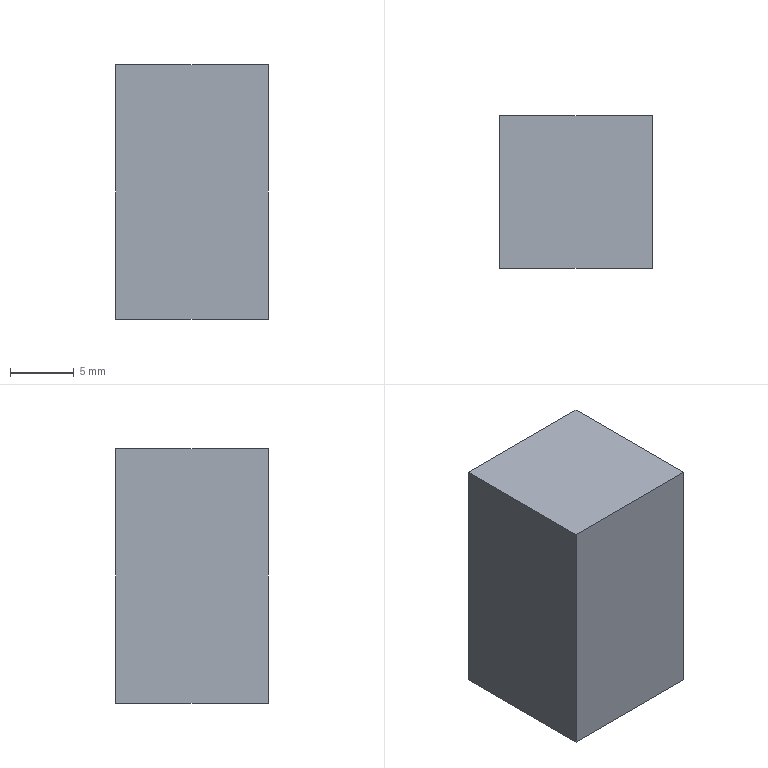Part | NX | features solid 2 | 1 solid | 6 faces | box 12 x 12 x 20 mm | volume 2880 mm3 | plane 6
STEP:
#1=CARTESIAN_POINT('',(-423.,722.,-30.));
#2=VERTEX_POINT('',#1);
#3=CARTESIAN_POINT('',(-423.,722.,-50.));
#4=VERTEX_POINT('',#3);
#5=CARTESIAN_POINT('',(-423.,722.,-30.));
#6=DIRECTION('',(0.,0.,1.));
#7=VECTOR('',#6,1000.);
#8=LINE('',#5,#7);
#9=EDGE_CURVE('',#2,#4,#8,.F.);
#10=ORIENTED_EDGE('',*,*,#9,.T.);
#11=CARTESIAN_POINT('',(-435.,722.,-50.));
#12=VERTEX_POINT('',#11);
#13=CARTESIAN_POINT('',(-435.,722.,-50.));
#14=DIRECTION('',(-1.,0.,0.));
#15=VECTOR('',#14,1000.);
#16=LINE('',#13,#15);
#17=EDGE_CURVE('',#12,#4,#16,.F.);
#18=ORIENTED_EDGE('',*,*,#17,.F.);
#19=CARTESIAN_POINT('',(-435.,722.,-30.));
#20=VERTEX_POINT('',#19);
#21=CARTESIAN_POINT('',(-435.,722.,-30.));
#22=DIRECTION('',(0.,0.,1.));
#23=VECTOR('',#22,1000.);
#24=LINE('',#21,#23);
#25=EDGE_CURVE('',#20,#12,#24,.F.);
#26=ORIENTED_EDGE('',*,*,#25,.F.);
#27=CARTESIAN_POINT('',(-435.,722.,-30.));
#28=DIRECTION('',(1.,0.,0.));
#29=VECTOR('',#28,1000.);
#30=LINE('',#27,#29);
#31=EDGE_CURVE('',#20,#2,#30,.T.);
#32=ORIENTED_EDGE('',*,*,#31,.T.);
#33=EDGE_LOOP('',(#10,#18,#26,#32));
#34=FACE_BOUND('',#33,.T.);
#35=CARTESIAN_POINT('',(-435.,722.,-30.));
#36=DIRECTION('',(0.,1.,0.));
#37=DIRECTION('',(1.,0.,0.));
#38=AXIS2_PLACEMENT_3D('',#35,#36,#37);
#39=PLANE('',#38);
#40=ADVANCED_FACE('',(#34),#39,.T.);
#41=ORIENTED_EDGE('',*,*,#25,.T.);
#42=CARTESIAN_POINT('',(-435.,710.,-50.));
#43=VERTEX_POINT('',#42);
#44=CARTESIAN_POINT('',(-435.,722.,-50.));
#45=DIRECTION('',(0.,1.,0.));
#46=VECTOR('',#45,1000.);
#47=LINE('',#44,#46);
#48=EDGE_CURVE('',#12,#43,#47,.F.);
#49=ORIENTED_EDGE('',*,*,#48,.T.);
#50=CARTESIAN_POINT('',(-435.,710.,-30.));
#51=VERTEX_POINT('',#50);
#52=CARTESIAN_POINT('',(-435.,710.,-30.));
#53=DIRECTION('',(0.,0.,1.));
#54=VECTOR('',#53,1000.);
#55=LINE('',#52,#54);
#56=EDGE_CURVE('',#51,#43,#55,.F.);
#57=ORIENTED_EDGE('',*,*,#56,.F.);
#58=CARTESIAN_POINT('',(-435.,722.,-30.));
#59=DIRECTION('',(0.,-1.,0.));
#60=VECTOR('',#59,1000.);
#61=LINE('',#58,#60);
#62=EDGE_CURVE('',#20,#51,#61,.T.);
#63=ORIENTED_EDGE('',*,*,#62,.F.);
#64=EDGE_LOOP('',(#41,#49,#57,#63));
#65=FACE_BOUND('',#64,.T.);
#66=CARTESIAN_POINT('',(-435.,722.,-30.));
#67=DIRECTION('',(1.,0.,0.));
#68=DIRECTION('',(0.,-1.,0.));
#69=AXIS2_PLACEMENT_3D('',#66,#67,#68);
#70=PLANE('',#69);
#71=ADVANCED_FACE('',(#65),#70,.F.);
#72=ORIENTED_EDGE('',*,*,#56,.T.);
#73=CARTESIAN_POINT('',(-423.,710.,-50.));
#74=VERTEX_POINT('',#73);
#75=CARTESIAN_POINT('',(-435.,710.,-50.));
#76=DIRECTION('',(-1.,0.,0.));
#77=VECTOR('',#76,1000.);
#78=LINE('',#75,#77);
#79=EDGE_CURVE('',#43,#74,#78,.F.);
#80=ORIENTED_EDGE('',*,*,#79,.T.);
#81=CARTESIAN_POINT('',(-423.,710.,-30.));
#82=VERTEX_POINT('',#81);
#83=CARTESIAN_POINT('',(-423.,710.,-30.));
#84=DIRECTION('',(0.,0.,1.));
#85=VECTOR('',#84,1000.);
#86=LINE('',#83,#85);
#87=EDGE_CURVE('',#82,#74,#86,.F.);
#88=ORIENTED_EDGE('',*,*,#87,.F.);
#89=CARTESIAN_POINT('',(-435.,710.,-30.));
#90=DIRECTION('',(1.,0.,0.));
#91=VECTOR('',#90,1000.);
#92=LINE('',#89,#91);
#93=EDGE_CURVE('',#51,#82,#92,.T.);
#94=ORIENTED_EDGE('',*,*,#93,.F.);
#95=EDGE_LOOP('',(#72,#80,#88,#94));
#96=FACE_BOUND('',#95,.T.);
#97=CARTESIAN_POINT('',(-435.,710.,-30.));
#98=DIRECTION('',(0.,1.,0.));
#99=DIRECTION('',(1.,0.,0.));
#100=AXIS2_PLACEMENT_3D('',#97,#98,#99);
#101=PLANE('',#100);
#102=ADVANCED_FACE('',(#96),#101,.F.);
#103=CARTESIAN_POINT('',(-423.,722.,-30.));
#104=DIRECTION('',(0.,-1.,0.));
#105=VECTOR('',#104,1000.);
#106=LINE('',#103,#105);
#107=EDGE_CURVE('',#2,#82,#106,.T.);
#108=ORIENTED_EDGE('',*,*,#107,.T.);
#109=ORIENTED_EDGE('',*,*,#87,.T.);
#110=CARTESIAN_POINT('',(-423.,722.,-50.));
#111=DIRECTION('',(0.,1.,0.));
#112=VECTOR('',#111,1000.);
#113=LINE('',#110,#112);
#114=EDGE_CURVE('',#4,#74,#113,.F.);
#115=ORIENTED_EDGE('',*,*,#114,.F.);
#116=ORIENTED_EDGE('',*,*,#9,.F.);
#117=EDGE_LOOP('',(#108,#109,#115,#116));
#118=FACE_BOUND('',#117,.T.);
#119=CARTESIAN_POINT('',(-423.,722.,-30.));
#120=DIRECTION('',(1.,0.,0.));
#121=DIRECTION('',(0.,-1.,0.));
#122=AXIS2_PLACEMENT_3D('',#119,#120,#121);
#123=PLANE('',#122);
#124=ADVANCED_FACE('',(#118),#123,.T.);
#125=ORIENTED_EDGE('',*,*,#79,.F.);
#126=ORIENTED_EDGE('',*,*,#48,.F.);
#127=ORIENTED_EDGE('',*,*,#17,.T.);
#128=ORIENTED_EDGE('',*,*,#114,.T.);
#129=EDGE_LOOP('',(#125,#126,#127,#128));
#130=FACE_BOUND('',#129,.T.);
#131=CARTESIAN_POINT('',(-435.,722.,-50.));
#132=DIRECTION('',(0.,0.,-1.));
#133=DIRECTION('',(-1.,0.,0.));
#134=AXIS2_PLACEMENT_3D('',#131,#132,#133);
#135=PLANE('',#134);
#136=ADVANCED_FACE('',(#130),#135,.T.);
#137=ORIENTED_EDGE('',*,*,#93,.T.);
#138=ORIENTED_EDGE('',*,*,#107,.F.);
#139=ORIENTED_EDGE('',*,*,#31,.F.);
#140=ORIENTED_EDGE('',*,*,#62,.T.);
#141=EDGE_LOOP('',(#137,#138,#139,#140));
#142=FACE_BOUND('',#141,.T.);
#143=CARTESIAN_POINT('',(-435.,722.,-30.));
#144=DIRECTION('',(0.,0.,-1.));
#145=DIRECTION('',(-1.,0.,0.));
#146=AXIS2_PLACEMENT_3D('',#143,#144,#145);
#147=PLANE('',#146);
#148=ADVANCED_FACE('',(#142),#147,.F.);
#149=CLOSED_SHELL('',(#40,#71,#102,#124,#136,#148));
#150=MANIFOLD_SOLID_BREP('',#149);
#151=(LENGTH_UNIT()NAMED_UNIT(*)SI_UNIT(.MILLI.,.METRE.));
#152=UNCERTAINTY_MEASURE_WITH_UNIT(LENGTH_MEASURE(0.00001),#151,'','');
#153=(NAMED_UNIT(*)PLANE_ANGLE_UNIT()SI_UNIT($,.RADIAN.));
#154=(NAMED_UNIT(*)SI_UNIT($,.STERADIAN.)SOLID_ANGLE_UNIT());
#155=(GEOMETRIC_REPRESENTATION_CONTEXT(3)GLOBAL_UNCERTAINTY_ASSIGNED_CONTEXT((#152))GLOBAL_UNIT_ASSIGNED_CONTEXT((#151,#153,#154))REPRESENTATION_CONTEXT('',''));
#156=ADVANCED_BREP_SHAPE_REPRESENTATION('',(#150),#155);